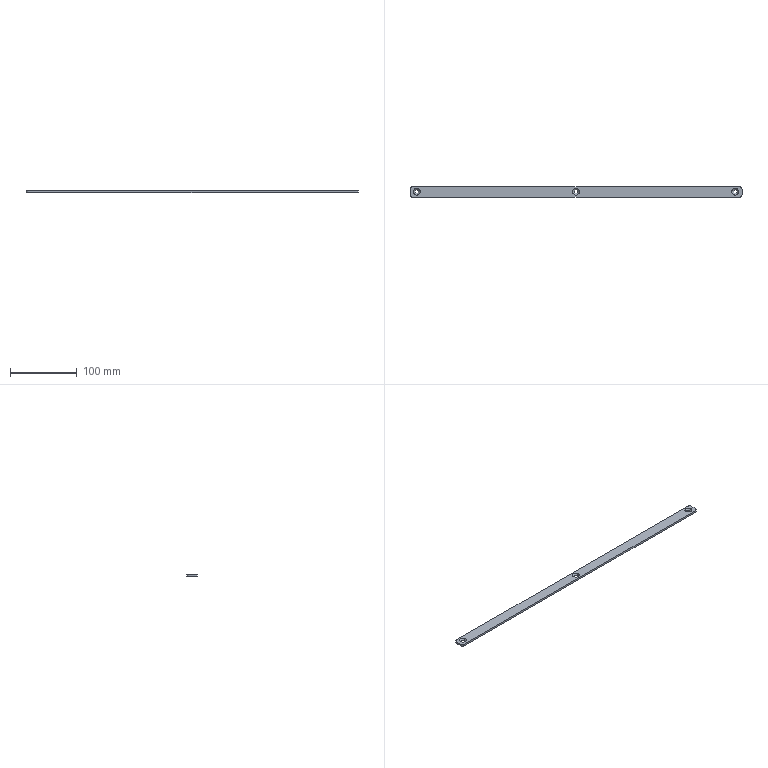Part | STEP file | 602-06-0016 | 1 solid | 22 faces | box 498 x 16 x 3 mm | volume 23447 mm3 | cylinder 10 | cone 6 | plane 6 | commonest cylinder face diameters 5.5 x6 8 x4